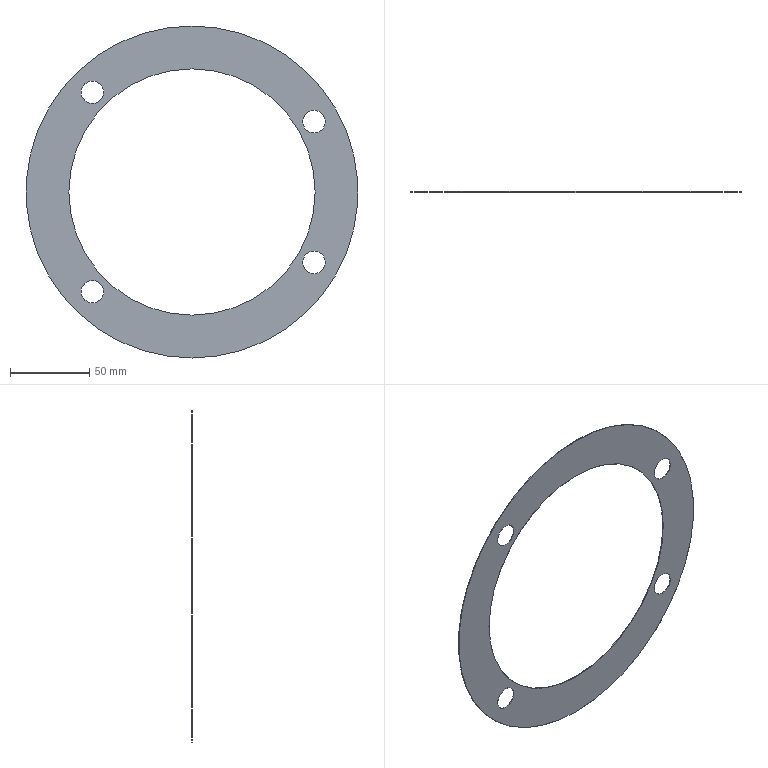Part | SolidWorks | features 3DProfileFeature 1, Extrusion 1, HoleWzd 1, MirrorPattern 1 | 1 solid | 14 faces | box 209.55 x 0.381 x 209.55 mm | volume 5665 mm3 | cylinder 12 | plane 2 | commonest cylinder face diameters 14.287 x8 155.448 x2 209.55 x2
STEP:
#1=CARTESIAN_POINT('',(-62.859,0.,55.721));
#2=VERTEX_POINT('',#1);
#3=CARTESIAN_POINT('',(-62.859,0.,70.009));
#4=VERTEX_POINT('',#3);
#5=CARTESIAN_POINT('',(-62.859,0.,62.865));
#6=DIRECTION('',(0.,1.,0.));
#7=DIRECTION('',(0.,0.,1.));
#8=AXIS2_PLACEMENT_3D('',#5,#6,#7);
#9=CIRCLE('',#8,7.144);
#10=EDGE_CURVE('',#2,#4,#9,.T.);
#11=ORIENTED_EDGE('',*,*,#10,.F.);
#12=CARTESIAN_POINT('',(-62.859,0.381,55.721));
#13=VERTEX_POINT('',#12);
#14=CARTESIAN_POINT('',(-62.859,0.381,55.721));
#15=DIRECTION('',(0.,1.,0.));
#16=VECTOR('',#15,1000.);
#17=LINE('',#14,#16);
#18=EDGE_CURVE('',#2,#13,#17,.T.);
#19=ORIENTED_EDGE('',*,*,#18,.T.);
#20=CARTESIAN_POINT('',(-62.859,0.381,70.009));
#21=VERTEX_POINT('',#20);
#22=CARTESIAN_POINT('',(-62.859,0.381,62.865));
#23=DIRECTION('',(0.,1.,0.));
#24=DIRECTION('',(0.,0.,1.));
#25=AXIS2_PLACEMENT_3D('',#22,#23,#24);
#26=CIRCLE('',#25,7.144);
#27=EDGE_CURVE('',#13,#21,#26,.T.);
#28=ORIENTED_EDGE('',*,*,#27,.T.);
#29=CARTESIAN_POINT('',(-62.859,0.381,70.009));
#30=DIRECTION('',(0.,1.,0.));
#31=VECTOR('',#30,1000.);
#32=LINE('',#29,#31);
#33=EDGE_CURVE('',#4,#21,#32,.T.);
#34=ORIENTED_EDGE('',*,*,#33,.F.);
#35=EDGE_LOOP('',(#11,#19,#28,#34));
#36=FACE_OUTER_BOUND('',#35,.T.);
#37=CARTESIAN_POINT('',(-62.859,0.381,62.865));
#38=DIRECTION('',(0.,1.,0.));
#39=DIRECTION('',(0.,0.,1.));
#40=AXIS2_PLACEMENT_3D('',#37,#38,#39);
#41=CYLINDRICAL_SURFACE('',#40,7.144);
#42=ADVANCED_FACE('',(#36),#41,.F.);
#43=CARTESIAN_POINT('',(76.987,0.,37.306));
#44=VERTEX_POINT('',#43);
#45=CARTESIAN_POINT('',(76.987,0.,51.594));
#46=VERTEX_POINT('',#45);
#47=CARTESIAN_POINT('',(76.987,0.,44.45));
#48=DIRECTION('',(0.,1.,0.));
#49=DIRECTION('',(0.,0.,1.));
#50=AXIS2_PLACEMENT_3D('',#47,#48,#49);
#51=CIRCLE('',#50,7.144);
#52=EDGE_CURVE('',#44,#46,#51,.T.);
#53=ORIENTED_EDGE('',*,*,#52,.F.);
#54=CARTESIAN_POINT('',(76.987,0.381,37.306));
#55=VERTEX_POINT('',#54);
#56=CARTESIAN_POINT('',(76.987,0.381,37.306));
#57=DIRECTION('',(0.,1.,0.));
#58=VECTOR('',#57,1000.);
#59=LINE('',#56,#58);
#60=EDGE_CURVE('',#44,#55,#59,.T.);
#61=ORIENTED_EDGE('',*,*,#60,.T.);
#62=CARTESIAN_POINT('',(76.987,0.381,51.594));
#63=VERTEX_POINT('',#62);
#64=CARTESIAN_POINT('',(76.987,0.381,44.45));
#65=DIRECTION('',(0.,1.,0.));
#66=DIRECTION('',(0.,0.,1.));
#67=AXIS2_PLACEMENT_3D('',#64,#65,#66);
#68=CIRCLE('',#67,7.144);
#69=EDGE_CURVE('',#55,#63,#68,.T.);
#70=ORIENTED_EDGE('',*,*,#69,.T.);
#71=CARTESIAN_POINT('',(76.987,0.381,51.594));
#72=DIRECTION('',(0.,1.,0.));
#73=VECTOR('',#72,1000.);
#74=LINE('',#71,#73);
#75=EDGE_CURVE('',#46,#63,#74,.T.);
#76=ORIENTED_EDGE('',*,*,#75,.F.);
#77=EDGE_LOOP('',(#53,#61,#70,#76));
#78=FACE_OUTER_BOUND('',#77,.T.);
#79=CARTESIAN_POINT('',(76.987,0.381,44.45));
#80=DIRECTION('',(0.,1.,0.));
#81=DIRECTION('',(0.,0.,1.));
#82=AXIS2_PLACEMENT_3D('',#79,#80,#81);
#83=CYLINDRICAL_SURFACE('',#82,7.144);
#84=ADVANCED_FACE('',(#78),#83,.F.);
#85=CARTESIAN_POINT('',(-62.859,0.,-70.009));
#86=VERTEX_POINT('',#85);
#87=CARTESIAN_POINT('',(-62.859,0.,-55.721));
#88=VERTEX_POINT('',#87);
#89=CARTESIAN_POINT('',(-62.859,0.,-62.865));
#90=DIRECTION('',(0.,1.,0.));
#91=DIRECTION('',(0.,0.,1.));
#92=AXIS2_PLACEMENT_3D('',#89,#90,#91);
#93=CIRCLE('',#92,7.144);
#94=EDGE_CURVE('',#86,#88,#93,.T.);
#95=ORIENTED_EDGE('',*,*,#94,.F.);
#96=CARTESIAN_POINT('',(-62.859,0.381,-70.009));
#97=VERTEX_POINT('',#96);
#98=CARTESIAN_POINT('',(-62.859,0.381,-70.009));
#99=DIRECTION('',(0.,1.,0.));
#100=VECTOR('',#99,1000.);
#101=LINE('',#98,#100);
#102=EDGE_CURVE('',#86,#97,#101,.T.);
#103=ORIENTED_EDGE('',*,*,#102,.T.);
#104=CARTESIAN_POINT('',(-62.859,0.381,-55.721));
#105=VERTEX_POINT('',#104);
#106=CARTESIAN_POINT('',(-62.859,0.381,-62.865));
#107=DIRECTION('',(0.,1.,0.));
#108=DIRECTION('',(0.,0.,1.));
#109=AXIS2_PLACEMENT_3D('',#106,#107,#108);
#110=CIRCLE('',#109,7.144);
#111=EDGE_CURVE('',#97,#105,#110,.T.);
#112=ORIENTED_EDGE('',*,*,#111,.T.);
#113=CARTESIAN_POINT('',(-62.859,0.381,-55.721));
#114=DIRECTION('',(0.,1.,0.));
#115=VECTOR('',#114,1000.);
#116=LINE('',#113,#115);
#117=EDGE_CURVE('',#88,#105,#116,.T.);
#118=ORIENTED_EDGE('',*,*,#117,.F.);
#119=EDGE_LOOP('',(#95,#103,#112,#118));
#120=FACE_OUTER_BOUND('',#119,.T.);
#121=CARTESIAN_POINT('',(-62.859,0.381,-62.865));
#122=DIRECTION('',(0.,1.,0.));
#123=DIRECTION('',(0.,0.,1.));
#124=AXIS2_PLACEMENT_3D('',#121,#122,#123);
#125=CYLINDRICAL_SURFACE('',#124,7.144);
#126=ADVANCED_FACE('',(#120),#125,.F.);
#127=CARTESIAN_POINT('',(76.987,0.,-51.594));
#128=VERTEX_POINT('',#127);
#129=CARTESIAN_POINT('',(76.987,0.,-37.306));
#130=VERTEX_POINT('',#129);
#131=CARTESIAN_POINT('',(76.987,0.,-44.45));
#132=DIRECTION('',(0.,1.,0.));
#133=DIRECTION('',(0.,0.,1.));
#134=AXIS2_PLACEMENT_3D('',#131,#132,#133);
#135=CIRCLE('',#134,7.144);
#136=EDGE_CURVE('',#128,#130,#135,.T.);
#137=ORIENTED_EDGE('',*,*,#136,.F.);
#138=CARTESIAN_POINT('',(76.987,0.381,-51.594));
#139=VERTEX_POINT('',#138);
#140=CARTESIAN_POINT('',(76.987,0.381,-51.594));
#141=DIRECTION('',(0.,1.,0.));
#142=VECTOR('',#141,1000.);
#143=LINE('',#140,#142);
#144=EDGE_CURVE('',#128,#139,#143,.T.);
#145=ORIENTED_EDGE('',*,*,#144,.T.);
#146=CARTESIAN_POINT('',(76.987,0.381,-37.306));
#147=VERTEX_POINT('',#146);
#148=CARTESIAN_POINT('',(76.987,0.381,-44.45));
#149=DIRECTION('',(0.,1.,0.));
#150=DIRECTION('',(0.,0.,1.));
#151=AXIS2_PLACEMENT_3D('',#148,#149,#150);
#152=CIRCLE('',#151,7.144);
#153=EDGE_CURVE('',#139,#147,#152,.T.);
#154=ORIENTED_EDGE('',*,*,#153,.T.);
#155=CARTESIAN_POINT('',(76.987,0.381,-37.306));
#156=DIRECTION('',(0.,1.,0.));
#157=VECTOR('',#156,1000.);
#158=LINE('',#155,#157);
#159=EDGE_CURVE('',#130,#147,#158,.T.);
#160=ORIENTED_EDGE('',*,*,#159,.F.);
#161=EDGE_LOOP('',(#137,#145,#154,#160));
#162=FACE_OUTER_BOUND('',#161,.T.);
#163=CARTESIAN_POINT('',(76.987,0.381,-44.45));
#164=DIRECTION('',(0.,1.,0.));
#165=DIRECTION('',(0.,0.,1.));
#166=AXIS2_PLACEMENT_3D('',#163,#164,#165);
#167=CYLINDRICAL_SURFACE('',#166,7.144);
#168=ADVANCED_FACE('',(#162),#167,.F.);
#169=CARTESIAN_POINT('',(0.,0.381,-77.724));
#170=VERTEX_POINT('',#169);
#171=CARTESIAN_POINT('',(0.,0.381,77.724));
#172=VERTEX_POINT('',#171);
#173=CARTESIAN_POINT('',(0.,0.381,0.));
#174=DIRECTION('',(0.,1.,0.));
#175=DIRECTION('',(0.,0.,1.));
#176=AXIS2_PLACEMENT_3D('',#173,#174,#175);
#177=CIRCLE('',#176,77.724);
#178=EDGE_CURVE('',#170,#172,#177,.T.);
#179=ORIENTED_EDGE('',*,*,#178,.T.);
#180=CARTESIAN_POINT('',(0.,0.,77.724));
#181=VERTEX_POINT('',#180);
#182=CARTESIAN_POINT('',(0.,0.381,77.724));
#183=DIRECTION('',(0.,-1.,0.));
#184=VECTOR('',#183,1000.);
#185=LINE('',#182,#184);
#186=EDGE_CURVE('',#172,#181,#185,.T.);
#187=ORIENTED_EDGE('',*,*,#186,.T.);
#188=CARTESIAN_POINT('',(0.,0.,-77.724));
#189=VERTEX_POINT('',#188);
#190=CARTESIAN_POINT('',(0.,0.,0.));
#191=DIRECTION('',(0.,1.,0.));
#192=DIRECTION('',(0.,0.,1.));
#193=AXIS2_PLACEMENT_3D('',#190,#191,#192);
#194=CIRCLE('',#193,77.724);
#195=EDGE_CURVE('',#189,#181,#194,.T.);
#196=ORIENTED_EDGE('',*,*,#195,.F.);
#197=CARTESIAN_POINT('',(0.,0.381,-77.724));
#198=DIRECTION('',(0.,-1.,0.));
#199=VECTOR('',#198,1000.);
#200=LINE('',#197,#199);
#201=EDGE_CURVE('',#170,#189,#200,.T.);
#202=ORIENTED_EDGE('',*,*,#201,.F.);
#203=EDGE_LOOP('',(#179,#187,#196,#202));
#204=FACE_OUTER_BOUND('',#203,.T.);
#205=CARTESIAN_POINT('',(0.,0.381,0.));
#206=DIRECTION('',(0.,-1.,0.));
#207=DIRECTION('',(0.,0.,-1.));
#208=AXIS2_PLACEMENT_3D('',#205,#206,#207);
#209=CYLINDRICAL_SURFACE('',#208,77.724);
#210=ADVANCED_FACE('',(#204),#209,.F.);
#211=CARTESIAN_POINT('',(0.,0.381,104.775));
#212=VERTEX_POINT('',#211);
#213=CARTESIAN_POINT('',(0.,0.381,-104.775));
#214=VERTEX_POINT('',#213);
#215=CARTESIAN_POINT('',(0.,0.381,0.));
#216=DIRECTION('',(0.,1.,0.));
#217=DIRECTION('',(0.,0.,1.));
#218=AXIS2_PLACEMENT_3D('',#215,#216,#217);
#219=CIRCLE('',#218,104.775);
#220=EDGE_CURVE('',#212,#214,#219,.T.);
#221=ORIENTED_EDGE('',*,*,#220,.F.);
#222=CARTESIAN_POINT('',(0.,0.,104.775));
#223=VERTEX_POINT('',#222);
#224=CARTESIAN_POINT('',(0.,0.381,104.775));
#225=DIRECTION('',(0.,-1.,0.));
#226=VECTOR('',#225,1000.);
#227=LINE('',#224,#226);
#228=EDGE_CURVE('',#212,#223,#227,.T.);
#229=ORIENTED_EDGE('',*,*,#228,.T.);
#230=CARTESIAN_POINT('',(0.,0.,-104.775));
#231=VERTEX_POINT('',#230);
#232=CARTESIAN_POINT('',(0.,0.,0.));
#233=DIRECTION('',(0.,1.,0.));
#234=DIRECTION('',(0.,0.,1.));
#235=AXIS2_PLACEMENT_3D('',#232,#233,#234);
#236=CIRCLE('',#235,104.775);
#237=EDGE_CURVE('',#223,#231,#236,.T.);
#238=ORIENTED_EDGE('',*,*,#237,.T.);
#239=CARTESIAN_POINT('',(0.,0.381,-104.775));
#240=DIRECTION('',(0.,-1.,0.));
#241=VECTOR('',#240,1000.);
#242=LINE('',#239,#241);
#243=EDGE_CURVE('',#214,#231,#242,.T.);
#244=ORIENTED_EDGE('',*,*,#243,.F.);
#245=EDGE_LOOP('',(#221,#229,#238,#244));
#246=FACE_OUTER_BOUND('',#245,.T.);
#247=CARTESIAN_POINT('',(0.,0.381,0.));
#248=DIRECTION('',(0.,-1.,0.));
#249=DIRECTION('',(0.,0.,-1.));
#250=AXIS2_PLACEMENT_3D('',#247,#248,#249);
#251=CYLINDRICAL_SURFACE('',#250,104.775);
#252=ADVANCED_FACE('',(#246),#251,.T.);
#253=CARTESIAN_POINT('',(-62.859,0.381,62.865));
#254=DIRECTION('',(0.,1.,0.));
#255=DIRECTION('',(0.,0.,1.));
#256=AXIS2_PLACEMENT_3D('',#253,#254,#255);
#257=CIRCLE('',#256,7.144);
#258=EDGE_CURVE('',#21,#13,#257,.T.);
#259=ORIENTED_EDGE('',*,*,#258,.F.);
#260=ORIENTED_EDGE('',*,*,#27,.F.);
#261=EDGE_LOOP('',(#259,#260));
#262=FACE_BOUND('',#261,.T.);
#263=CARTESIAN_POINT('',(76.987,0.381,44.45));
#264=DIRECTION('',(0.,1.,0.));
#265=DIRECTION('',(0.,0.,1.));
#266=AXIS2_PLACEMENT_3D('',#263,#264,#265);
#267=CIRCLE('',#266,7.144);
#268=EDGE_CURVE('',#63,#55,#267,.T.);
#269=ORIENTED_EDGE('',*,*,#268,.F.);
#270=ORIENTED_EDGE('',*,*,#69,.F.);
#271=EDGE_LOOP('',(#269,#270));
#272=FACE_BOUND('',#271,.T.);
#273=CARTESIAN_POINT('',(-62.859,0.381,-62.865));
#274=DIRECTION('',(0.,1.,0.));
#275=DIRECTION('',(0.,0.,1.));
#276=AXIS2_PLACEMENT_3D('',#273,#274,#275);
#277=CIRCLE('',#276,7.144);
#278=EDGE_CURVE('',#105,#97,#277,.T.);
#279=ORIENTED_EDGE('',*,*,#278,.F.);
#280=ORIENTED_EDGE('',*,*,#111,.F.);
#281=EDGE_LOOP('',(#279,#280));
#282=FACE_BOUND('',#281,.T.);
#283=CARTESIAN_POINT('',(76.987,0.381,-44.45));
#284=DIRECTION('',(0.,1.,0.));
#285=DIRECTION('',(0.,0.,1.));
#286=AXIS2_PLACEMENT_3D('',#283,#284,#285);
#287=CIRCLE('',#286,7.144);
#288=EDGE_CURVE('',#147,#139,#287,.T.);
#289=ORIENTED_EDGE('',*,*,#288,.F.);
#290=ORIENTED_EDGE('',*,*,#153,.F.);
#291=EDGE_LOOP('',(#289,#290));
#292=FACE_BOUND('',#291,.T.);
#293=CARTESIAN_POINT('',(0.,0.381,0.));
#294=DIRECTION('',(0.,1.,0.));
#295=DIRECTION('',(0.,0.,1.));
#296=AXIS2_PLACEMENT_3D('',#293,#294,#295);
#297=CIRCLE('',#296,104.775);
#298=EDGE_CURVE('',#214,#212,#297,.T.);
#299=ORIENTED_EDGE('',*,*,#298,.T.);
#300=ORIENTED_EDGE('',*,*,#220,.T.);
#301=EDGE_LOOP('',(#299,#300));
#302=FACE_OUTER_BOUND('',#301,.T.);
#303=ORIENTED_EDGE('',*,*,#178,.F.);
#304=CARTESIAN_POINT('',(0.,0.381,0.));
#305=DIRECTION('',(0.,1.,0.));
#306=DIRECTION('',(0.,0.,1.));
#307=AXIS2_PLACEMENT_3D('',#304,#305,#306);
#308=CIRCLE('',#307,77.724);
#309=EDGE_CURVE('',#172,#170,#308,.T.);
#310=ORIENTED_EDGE('',*,*,#309,.F.);
#311=EDGE_LOOP('',(#303,#310));
#312=FACE_BOUND('',#311,.T.);
#313=CARTESIAN_POINT('',(0.,0.381,0.));
#314=DIRECTION('',(0.,1.,0.));
#315=DIRECTION('',(0.,0.,1.));
#316=AXIS2_PLACEMENT_3D('',#313,#314,#315);
#317=PLANE('',#316);
#318=ADVANCED_FACE('',(#262,#272,#282,#292,#302,#312),#317,.T.);
#319=CARTESIAN_POINT('',(-62.859,0.,62.865));
#320=DIRECTION('',(0.,1.,0.));
#321=DIRECTION('',(0.,0.,1.));
#322=AXIS2_PLACEMENT_3D('',#319,#320,#321);
#323=CIRCLE('',#322,7.144);
#324=EDGE_CURVE('',#4,#2,#323,.T.);
#325=ORIENTED_EDGE('',*,*,#324,.T.);
#326=ORIENTED_EDGE('',*,*,#10,.T.);
#327=EDGE_LOOP('',(#325,#326));
#328=FACE_BOUND('',#327,.T.);
#329=CARTESIAN_POINT('',(76.987,0.,44.45));
#330=DIRECTION('',(0.,1.,0.));
#331=DIRECTION('',(0.,0.,1.));
#332=AXIS2_PLACEMENT_3D('',#329,#330,#331);
#333=CIRCLE('',#332,7.144);
#334=EDGE_CURVE('',#46,#44,#333,.T.);
#335=ORIENTED_EDGE('',*,*,#334,.T.);
#336=ORIENTED_EDGE('',*,*,#52,.T.);
#337=EDGE_LOOP('',(#335,#336));
#338=FACE_BOUND('',#337,.T.);
#339=CARTESIAN_POINT('',(-62.859,0.,-62.865));
#340=DIRECTION('',(0.,1.,0.));
#341=DIRECTION('',(0.,0.,1.));
#342=AXIS2_PLACEMENT_3D('',#339,#340,#341);
#343=CIRCLE('',#342,7.144);
#344=EDGE_CURVE('',#88,#86,#343,.T.);
#345=ORIENTED_EDGE('',*,*,#344,.T.);
#346=ORIENTED_EDGE('',*,*,#94,.T.);
#347=EDGE_LOOP('',(#345,#346));
#348=FACE_BOUND('',#347,.T.);
#349=CARTESIAN_POINT('',(76.987,0.,-44.45));
#350=DIRECTION('',(0.,1.,0.));
#351=DIRECTION('',(0.,0.,1.));
#352=AXIS2_PLACEMENT_3D('',#349,#350,#351);
#353=CIRCLE('',#352,7.144);
#354=EDGE_CURVE('',#130,#128,#353,.T.);
#355=ORIENTED_EDGE('',*,*,#354,.T.);
#356=ORIENTED_EDGE('',*,*,#136,.T.);
#357=EDGE_LOOP('',(#355,#356));
#358=FACE_BOUND('',#357,.T.);
#359=CARTESIAN_POINT('',(0.,0.,0.));
#360=DIRECTION('',(0.,1.,0.));
#361=DIRECTION('',(0.,0.,1.));
#362=AXIS2_PLACEMENT_3D('',#359,#360,#361);
#363=CIRCLE('',#362,104.775);
#364=EDGE_CURVE('',#231,#223,#363,.T.);
#365=ORIENTED_EDGE('',*,*,#364,.F.);
#366=ORIENTED_EDGE('',*,*,#237,.F.);
#367=EDGE_LOOP('',(#365,#366));
#368=FACE_OUTER_BOUND('',#367,.T.);
#369=ORIENTED_EDGE('',*,*,#195,.T.);
#370=CARTESIAN_POINT('',(0.,0.,0.));
#371=DIRECTION('',(0.,1.,0.));
#372=DIRECTION('',(0.,0.,1.));
#373=AXIS2_PLACEMENT_3D('',#370,#371,#372);
#374=CIRCLE('',#373,77.724);
#375=EDGE_CURVE('',#181,#189,#374,.T.);
#376=ORIENTED_EDGE('',*,*,#375,.T.);
#377=EDGE_LOOP('',(#369,#376));
#378=FACE_BOUND('',#377,.T.);
#379=CARTESIAN_POINT('',(0.,0.,0.));
#380=DIRECTION('',(0.,1.,0.));
#381=DIRECTION('',(0.,0.,1.));
#382=AXIS2_PLACEMENT_3D('',#379,#380,#381);
#383=PLANE('',#382);
#384=ADVANCED_FACE('',(#328,#338,#348,#358,#368,#378),#383,.F.);
#385=ORIENTED_EDGE('',*,*,#228,.F.);
#386=ORIENTED_EDGE('',*,*,#298,.F.);
#387=ORIENTED_EDGE('',*,*,#243,.T.);
#388=ORIENTED_EDGE('',*,*,#364,.T.);
#389=EDGE_LOOP('',(#385,#386,#387,#388));
#390=FACE_OUTER_BOUND('',#389,.T.);
#391=CARTESIAN_POINT('',(0.,0.381,0.));
#392=DIRECTION('',(0.,-1.,0.));
#393=DIRECTION('',(0.,0.,-1.));
#394=AXIS2_PLACEMENT_3D('',#391,#392,#393);
#395=CYLINDRICAL_SURFACE('',#394,104.775);
#396=ADVANCED_FACE('',(#390),#395,.T.);
#397=ORIENTED_EDGE('',*,*,#186,.F.);
#398=ORIENTED_EDGE('',*,*,#309,.T.);
#399=ORIENTED_EDGE('',*,*,#201,.T.);
#400=ORIENTED_EDGE('',*,*,#375,.F.);
#401=EDGE_LOOP('',(#397,#398,#399,#400));
#402=FACE_OUTER_BOUND('',#401,.T.);
#403=CARTESIAN_POINT('',(0.,0.381,0.));
#404=DIRECTION('',(0.,-1.,0.));
#405=DIRECTION('',(0.,0.,-1.));
#406=AXIS2_PLACEMENT_3D('',#403,#404,#405);
#407=CYLINDRICAL_SURFACE('',#406,77.724);
#408=ADVANCED_FACE('',(#402),#407,.F.);
#409=ORIENTED_EDGE('',*,*,#144,.F.);
#410=ORIENTED_EDGE('',*,*,#354,.F.);
#411=ORIENTED_EDGE('',*,*,#159,.T.);
#412=ORIENTED_EDGE('',*,*,#288,.T.);
#413=EDGE_LOOP('',(#409,#410,#411,#412));
#414=FACE_OUTER_BOUND('',#413,.T.);
#415=CARTESIAN_POINT('',(76.987,0.381,-44.45));
#416=DIRECTION('',(0.,1.,0.));
#417=DIRECTION('',(0.,0.,1.));
#418=AXIS2_PLACEMENT_3D('',#415,#416,#417);
#419=CYLINDRICAL_SURFACE('',#418,7.144);
#420=ADVANCED_FACE('',(#414),#419,.F.);
#421=ORIENTED_EDGE('',*,*,#102,.F.);
#422=ORIENTED_EDGE('',*,*,#344,.F.);
#423=ORIENTED_EDGE('',*,*,#117,.T.);
#424=ORIENTED_EDGE('',*,*,#278,.T.);
#425=EDGE_LOOP('',(#421,#422,#423,#424));
#426=FACE_OUTER_BOUND('',#425,.T.);
#427=CARTESIAN_POINT('',(-62.859,0.381,-62.865));
#428=DIRECTION('',(0.,1.,0.));
#429=DIRECTION('',(0.,0.,1.));
#430=AXIS2_PLACEMENT_3D('',#427,#428,#429);
#431=CYLINDRICAL_SURFACE('',#430,7.144);
#432=ADVANCED_FACE('',(#426),#431,.F.);
#433=ORIENTED_EDGE('',*,*,#60,.F.);
#434=ORIENTED_EDGE('',*,*,#334,.F.);
#435=ORIENTED_EDGE('',*,*,#75,.T.);
#436=ORIENTED_EDGE('',*,*,#268,.T.);
#437=EDGE_LOOP('',(#433,#434,#435,#436));
#438=FACE_OUTER_BOUND('',#437,.T.);
#439=CARTESIAN_POINT('',(76.987,0.381,44.45));
#440=DIRECTION('',(0.,1.,0.));
#441=DIRECTION('',(0.,0.,1.));
#442=AXIS2_PLACEMENT_3D('',#439,#440,#441);
#443=CYLINDRICAL_SURFACE('',#442,7.144);
#444=ADVANCED_FACE('',(#438),#443,.F.);
#445=ORIENTED_EDGE('',*,*,#18,.F.);
#446=ORIENTED_EDGE('',*,*,#324,.F.);
#447=ORIENTED_EDGE('',*,*,#33,.T.);
#448=ORIENTED_EDGE('',*,*,#258,.T.);
#449=EDGE_LOOP('',(#445,#446,#447,#448));
#450=FACE_OUTER_BOUND('',#449,.T.);
#451=CARTESIAN_POINT('',(-62.859,0.381,62.865));
#452=DIRECTION('',(0.,1.,0.));
#453=DIRECTION('',(0.,0.,1.));
#454=AXIS2_PLACEMENT_3D('',#451,#452,#453);
#455=CYLINDRICAL_SURFACE('',#454,7.144);
#456=ADVANCED_FACE('',(#450),#455,.F.);
#457=CLOSED_SHELL('',(#42,#84,#126,#168,#210,#252,#318,#384,#396,#408,#420,#432,#444,#456));
#458=MANIFOLD_SOLID_BREP('',#457);
#459=CARTESIAN_POINT('',(0.,0.,0.));
#460=DIRECTION('',(0.,0.,1.));
#461=DIRECTION('',(1.,0.,0.));
#462=AXIS2_PLACEMENT_3D('',#459,#460,#461);
#463=(LENGTH_UNIT()NAMED_UNIT(*)SI_UNIT(.MILLI.,.METRE.));
#464=UNCERTAINTY_MEASURE_WITH_UNIT(LENGTH_MEASURE(0.00001),#463,'','');
#465=(NAMED_UNIT(*)PLANE_ANGLE_UNIT()SI_UNIT($,.RADIAN.));
#466=(NAMED_UNIT(*)SI_UNIT($,.STERADIAN.)SOLID_ANGLE_UNIT());
#467=(GEOMETRIC_REPRESENTATION_CONTEXT(3)GLOBAL_UNCERTAINTY_ASSIGNED_CONTEXT((#464))GLOBAL_UNIT_ASSIGNED_CONTEXT((#463,#465,#466))REPRESENTATION_CONTEXT('',''));
#468=ADVANCED_BREP_SHAPE_REPRESENTATION('',(#458,#462),#467);